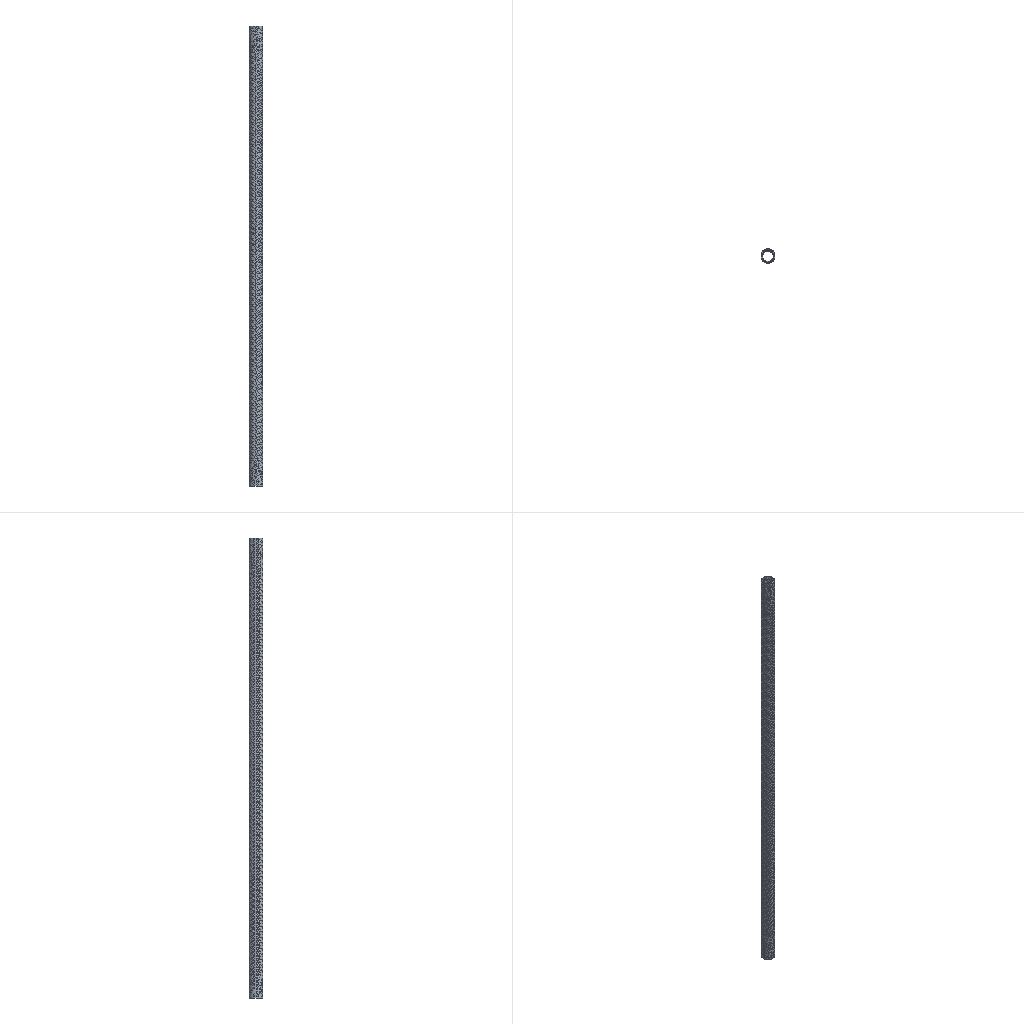Simulation study | ansys workbench
Ansys APDL input file, long lists of numbers shortened:
/batch
/config,noeldb,1     ! force off writing results to database
*get,_wallstrt,active,,time,wall
! ANSYS input file written by Workbench version 2022 R1
! File used for geometry attach: F:\ansys（分析文件汇总)\ansys刀片有限元分析\装配体\长杆.STEP
/title,2222--____ (D5)
! ****** Begin Custom Load Command Snippet ******
/COM, ACT Extensions:
/COM,     LSDYNA, 2021.1
/COM,
! ****** End   Custom Load Command Snippet ******
*DIM,_wb_ProjectScratch_dir,string,248
_wb_ProjectScratch_dir(1) = 'F:\ansys（分析文件汇总)\ansys刀片有限元分析\_ProjectScratch\ScrB55E\'
*DIM,_wb_SolverFiles_dir,string,248
_wb_SolverFiles_dir(1) = 'F:\ansys（分析文件汇总)\ansys刀片有限元分析\2222_files\dp0\SYS-2\MECH\'
*DIM,_wb_userfiles_dir,string,248
_wb_userfiles_dir(1) = 'F:\ansys（分析文件汇总)\ansys刀片有限元分析\2222_files\user_files\'
/com,--- Data in consistent NMM units. See Solving Units in the help system for more information.
/units,MPA
/nopr
/wb,file,start              !  signify a WB generated input file
/prep7
! Turn off shape checking because checks already performed inside WB mesher.
! See help system for more information.
SHPP,OFF,,NOWARN
/nolist
etcon,set             ! allow ANSYS to choose best KEYOP's for 180x elements, resets any applicable keyopt to MAPDL defaults
/com,*********** Nodes for the whole assembly ***********
nblock,3,,27396
(1i9,3e20.9e3)
        1     2.250000000E+01     2.755455298E-15    -2.500000000E+02
! (24905 more lines like these left out)
-1
/com,*********** Nodes for all Remote Points ***********
nblock,3
(1i9,3e20.9e3)
    24907    -5.505508782E-16     1.776356839E-15    -1.000000000E+03
-1
/wb,elem,start            !  set before creation of elements
/com,*********** Elements for Body 1 "__-FreeParts|__-__1" ***********
et,1,187
eblock,19,solid,,12612
(19i9)
        1        1        1        1        0        0        0        0       10        0        1       13     1910     1747     3535     4192    16252     4190     4196
! (25223 more lines like these left out)
-1
/wb,elem,end               !  done creating elements
/com,*********** Send User Defined Coordinate System(s) ***********
csys,0
toffst,273.15,  ! Temperature offset from absolute zero
/com,*********** Set Reference Temperature ***********
tref,22.
/wb,mat,start              !  starting to send materials
/com,*********** Send Materials ***********
Temperature = 'TEMP' ! Temperature
MP,DENS,1,7.85e-09,	! tonne mm^-3
MP,ALPX,1,1.2e-05,	! C^-1
MP,C,1,434000000,	! mm^2 s^-2 C^-1
MP,KXX,1,60.5,	! tonne mm s^-3 C^-1
MP,RSVX,1,0.00017,	! ohm mm
MP,EX,1,200000,	! tonne s^-2 mm^-1
MP,NUXY,1,0.3,
MP,MURX,1,10000,
/wb,mat,end                !  done sending materials
!************************* Model Summary ********************
!__-FreeParts|__-__1,	结构钢,	matid,	1
!************************* End Model Summary ********************
! get the diagonal of the bounding box. Needed later for other things
*get,_xmin,node,,mnloc,x
*get,_ymin,node,,mnloc,y
*get,_zmin,node,,mnloc,z
*get,_xmax,node,,mxloc,x
*get,_ymax,node,,mxloc,y
*get,_zmax,node,,mxloc,z
_ASMDIAG=(_xmax-_xmin)*(_xmax-_xmin)+(_ymax-_ymin)*(_ymax-_ymin)+(_zmax-_zmin)*(_zmax-_zmin)
_ASMDIAG=SQRT(_ASMDIAG)
/wb,contact,start          !  starting to send contact
/wb,contact,end            !  done creating contacts
/golist
/wb,load,start             !  starting to send loads
/com,*********** Fixed Supports ***********
CMBLOCK,_FIXEDSU,NODE,      192
(8i10)
         1         2         3         4         5         6         7         8
! (23 more lines like these left out)
cmsel,s,_FIXEDSU
d,all,all
nsel,all
/com,*********** Create Remote Point "内部远程点" ***********
! -------- Remote Point Used by "力矩" --------
*set,tid,3
*set,cid,2
et,cid,174
et,tid,170
keyo,tid,2,1               ! Don't fix the pilot node
keyo,tid,4,111111
keyo,cid,12,5              ! Bonded Contact
keyo,cid,4,1               ! Deformable RBE3 style load
keyo,cid,2,2               ! MPC style contact
eblock,10,,,3908
(15i9)
    20782        2        2        2        0     2692      278     2860     2860     6454     6455     2860    21415
! (3907 more lines like these left out)
-1
*set,_npilot,24907
_npilot32=_npilot
type,tid
mat ,cid
real,cid
tshape,pilo
en,24690,_npilot
tshape
/com,*********** Construct Moment Using Remote Attachment ***********
/gst,on,on
fini
*get,_numnode,node,0,count
*get,_numelem,elem,0,count
*get, _MAXELEMNUM, elem, 0, NUM, MAX
*get, _MAXNODENUM, node, 0, NUM, MAX
*get, _MAXELEMTYPE, etyp, 0, NUM, MAX
*get, _MAXREALCONST, real, 0, NUM, MAX
/go
/wb,load,end               !  done creating loads
/com,--- Number of total nodes = %_numnode%
/com,--- Number of contact elements = 3908
/com,--- Number of spring elements = 0
/com,--- Number of bearing elements = 0
/com,--- Number of solid elements = 12612
/com,--- Number of condensed parts = 0
/com,--- Number of total elements = %_numelem%
*get,_wallbsol,active,,time,wall
/com,****************************************************************************
/com,*************************    SOLUTION       ********************************
/com,****************************************************************************
/solu
antype,0                   ! static analysis
_thickRatio=  0     ! Ratio of thick parts in the model
eqsl,sparse,,,,,1
cntr,print,1               ! print out contact info and also make no initial contact an error
dmpoption,emat,no             ! Don't combine emat file for DANSYS
dmpoption,esav,no             ! Don't combine esav file for DANSYS
nldiag,cont,iter           ! print out contact info each equilibrium iteration
rescontrol,,none                 ! Do not keep any restart files
/com,****************************************************
/com,******************* SOLVE FOR LS 1 OF 1 ****************
nsel,s,node,,24907
f,all,mx,0.
f,all,my,0.
f,all,mz,800000.
nsel,all
/nopr
/gopr
nsub,1,1,1
time,1.
outres,erase
outres,all,none
outres,nsol,all,
outres,rsol,all
outres,eangl,all
outres,etmp,all
outres,veng,all
outres,strs,all,
outres,epel,all,
outres,eppl,all,
outres,cont,all,
! *********** WB SOLVE COMMAND ***********
! check interactive state
*get,ANSINTER_,active,,int
*if,ANSINTER_,ne,0,then
/eof
*endif
solve
/com *************** Write FE CONNECTORS *********
CEWRITE,file,ce,,INTE
/com,****************************************************
/com,*************** FINISHED SOLVE FOR LS 1 *************
*get,_wallasol,active,,time,wall
/nopr
*get,_numnode,node,0,count
*get,_numelem,elem,0,count
*get, _MAXELEMNUM, elem, 0, NUM, MAX
*get, _MAXNODENUM, node, 0, NUM, MAX,,,INTERNAL
*get, _MAXELEMTYPE, etyp, 0, NUM, MAX
*get, _MAXREALCONST, real, 0, NUM, MAX
/gopr
/post1
xmlo,ENCODING,ISO-8859-1
xmlo,parm
/xml,parm,xml
fini
/gopr
*get,_walldone,active,,time,wall
_preptime=(_wallbsol-_wallstrt)*3600
_solvtime=(_wallasol-_wallbsol)*3600
_posttime=(_walldone-_wallasol)*3600
_totaltim=(_walldone-_wallstrt)*3600
*get,_dlbratio,active,0,solu,dlbr
*get,_combtime,active,0,solu,comb
*get,_ssmode,active,0,solu,ssmm
*get,_ndofs,active,0,solu,ndof
*get,_sol_end_time,active,0,set,time
*if,_sol_end_time,eq,1.,then
/fclean				!clean distributed files
*endif
/com,--- Total number of nodes = %_numnode%
/com,--- Total number of elements = %_numelem%
/com,--- Element load balance ratio = %_dlbratio%
/com,--- Time to combine distributed files = %_combtime%
/com,--- Sparse memory mode = %_ssmode%
/com,--- Number of DOF = %_ndofs%
/wb,file,end               ! done with WB generated input